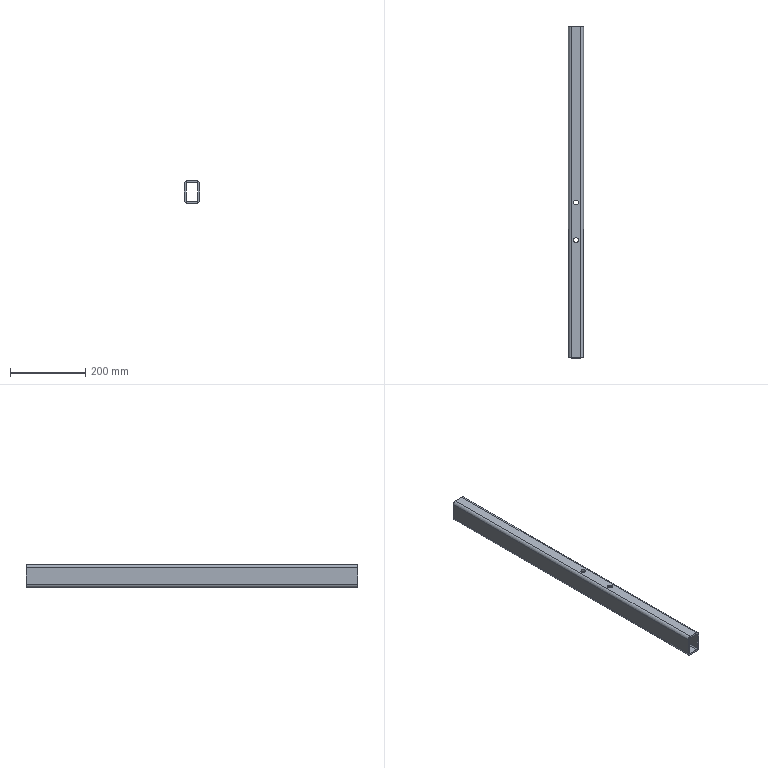Part | SolidWorks | features HoleWzd 1, WeldMemberFeat 1, WeldmentFeature 1 | 1 solid | 26 faces | box 40 x 884 x 60 mm | volume 751210 mm3 | cylinder 16 | plane 10 | commonest cylinder face diameters 13 x8 6 x4 16 x4
STEP:
#1=CARTESIAN_POINT('',(-6.5,314.,-30.));
#2=VERTEX_POINT('',#1);
#3=CARTESIAN_POINT('',(6.5,314.,-30.));
#4=VERTEX_POINT('',#3);
#5=CARTESIAN_POINT('',(0.,314.,-30.));
#6=DIRECTION('',(0.,0.,1.));
#7=DIRECTION('',(1.,0.,0.));
#8=AXIS2_PLACEMENT_3D('',#5,#6,#7);
#9=CIRCLE('',#8,6.5);
#10=EDGE_CURVE('',#2,#4,#9,.T.);
#11=ORIENTED_EDGE('',*,*,#10,.F.);
#12=CARTESIAN_POINT('',(-6.5,314.,-25.));
#13=VERTEX_POINT('',#12);
#14=CARTESIAN_POINT('',(-6.5,314.,30.));
#15=DIRECTION('',(0.,0.,1.));
#16=VECTOR('',#15,1000.);
#17=LINE('',#14,#16);
#18=EDGE_CURVE('',#2,#13,#17,.T.);
#19=ORIENTED_EDGE('',*,*,#18,.T.);
#20=CARTESIAN_POINT('',(6.5,314.,-25.));
#21=VERTEX_POINT('',#20);
#22=CARTESIAN_POINT('',(0.,314.,-25.));
#23=DIRECTION('',(0.,0.,1.));
#24=DIRECTION('',(1.,0.,0.));
#25=AXIS2_PLACEMENT_3D('',#22,#23,#24);
#26=CIRCLE('',#25,6.5);
#27=EDGE_CURVE('',#13,#21,#26,.T.);
#28=ORIENTED_EDGE('',*,*,#27,.T.);
#29=CARTESIAN_POINT('',(6.5,314.,30.));
#30=DIRECTION('',(0.,0.,1.));
#31=VECTOR('',#30,1000.);
#32=LINE('',#29,#31);
#33=EDGE_CURVE('',#4,#21,#32,.T.);
#34=ORIENTED_EDGE('',*,*,#33,.F.);
#35=EDGE_LOOP('',(#11,#19,#28,#34));
#36=FACE_OUTER_BOUND('',#35,.T.);
#37=CARTESIAN_POINT('',(0.,314.,30.));
#38=DIRECTION('',(0.,0.,1.));
#39=DIRECTION('',(1.,0.,0.));
#40=AXIS2_PLACEMENT_3D('',#37,#38,#39);
#41=CYLINDRICAL_SURFACE('',#40,6.5);
#42=ADVANCED_FACE('',(#36),#41,.F.);
#43=CARTESIAN_POINT('',(6.5,314.,25.));
#44=VERTEX_POINT('',#43);
#45=CARTESIAN_POINT('',(-6.5,314.,25.));
#46=VERTEX_POINT('',#45);
#47=CARTESIAN_POINT('',(0.,314.,25.));
#48=DIRECTION('',(0.,0.,-1.));
#49=DIRECTION('',(-1.,0.,0.));
#50=AXIS2_PLACEMENT_3D('',#47,#48,#49);
#51=CIRCLE('',#50,6.5);
#52=EDGE_CURVE('',#44,#46,#51,.T.);
#53=ORIENTED_EDGE('',*,*,#52,.T.);
#54=CARTESIAN_POINT('',(-6.5,314.,30.));
#55=VERTEX_POINT('',#54);
#56=CARTESIAN_POINT('',(-6.5,314.,30.));
#57=DIRECTION('',(0.,0.,1.));
#58=VECTOR('',#57,1000.);
#59=LINE('',#56,#58);
#60=EDGE_CURVE('',#46,#55,#59,.T.);
#61=ORIENTED_EDGE('',*,*,#60,.T.);
#62=CARTESIAN_POINT('',(6.5,314.,30.));
#63=VERTEX_POINT('',#62);
#64=CARTESIAN_POINT('',(0.,314.,30.));
#65=DIRECTION('',(0.,0.,1.));
#66=DIRECTION('',(1.,0.,0.));
#67=AXIS2_PLACEMENT_3D('',#64,#65,#66);
#68=CIRCLE('',#67,6.5);
#69=EDGE_CURVE('',#55,#63,#68,.T.);
#70=ORIENTED_EDGE('',*,*,#69,.T.);
#71=CARTESIAN_POINT('',(6.5,314.,30.));
#72=DIRECTION('',(0.,0.,1.));
#73=VECTOR('',#72,1000.);
#74=LINE('',#71,#73);
#75=EDGE_CURVE('',#44,#63,#74,.T.);
#76=ORIENTED_EDGE('',*,*,#75,.F.);
#77=EDGE_LOOP('',(#53,#61,#70,#76));
#78=FACE_OUTER_BOUND('',#77,.T.);
#79=CARTESIAN_POINT('',(0.,314.,30.));
#80=DIRECTION('',(0.,0.,1.));
#81=DIRECTION('',(1.,0.,0.));
#82=AXIS2_PLACEMENT_3D('',#79,#80,#81);
#83=CYLINDRICAL_SURFACE('',#82,6.5);
#84=ADVANCED_FACE('',(#78),#83,.F.);
#85=CARTESIAN_POINT('',(6.5,414.,25.));
#86=VERTEX_POINT('',#85);
#87=CARTESIAN_POINT('',(-6.5,414.,25.));
#88=VERTEX_POINT('',#87);
#89=CARTESIAN_POINT('',(0.,414.,25.));
#90=DIRECTION('',(0.,0.,-1.));
#91=DIRECTION('',(-1.,0.,0.));
#92=AXIS2_PLACEMENT_3D('',#89,#90,#91);
#93=CIRCLE('',#92,6.5);
#94=EDGE_CURVE('',#86,#88,#93,.T.);
#95=ORIENTED_EDGE('',*,*,#94,.T.);
#96=CARTESIAN_POINT('',(-6.5,414.,30.));
#97=VERTEX_POINT('',#96);
#98=CARTESIAN_POINT('',(-6.5,414.,30.));
#99=DIRECTION('',(0.,0.,1.));
#100=VECTOR('',#99,1000.);
#101=LINE('',#98,#100);
#102=EDGE_CURVE('',#88,#97,#101,.T.);
#103=ORIENTED_EDGE('',*,*,#102,.T.);
#104=CARTESIAN_POINT('',(6.5,414.,30.));
#105=VERTEX_POINT('',#104);
#106=CARTESIAN_POINT('',(0.,414.,30.));
#107=DIRECTION('',(0.,0.,1.));
#108=DIRECTION('',(1.,0.,0.));
#109=AXIS2_PLACEMENT_3D('',#106,#107,#108);
#110=CIRCLE('',#109,6.5);
#111=EDGE_CURVE('',#97,#105,#110,.T.);
#112=ORIENTED_EDGE('',*,*,#111,.T.);
#113=CARTESIAN_POINT('',(6.5,414.,30.));
#114=DIRECTION('',(0.,0.,1.));
#115=VECTOR('',#114,1000.);
#116=LINE('',#113,#115);
#117=EDGE_CURVE('',#86,#105,#116,.T.);
#118=ORIENTED_EDGE('',*,*,#117,.F.);
#119=EDGE_LOOP('',(#95,#103,#112,#118));
#120=FACE_OUTER_BOUND('',#119,.T.);
#121=CARTESIAN_POINT('',(0.,414.,30.));
#122=DIRECTION('',(0.,0.,1.));
#123=DIRECTION('',(1.,0.,0.));
#124=AXIS2_PLACEMENT_3D('',#121,#122,#123);
#125=CYLINDRICAL_SURFACE('',#124,6.5);
#126=ADVANCED_FACE('',(#120),#125,.F.);
#127=CARTESIAN_POINT('',(-6.5,414.,-30.));
#128=VERTEX_POINT('',#127);
#129=CARTESIAN_POINT('',(6.5,414.,-30.));
#130=VERTEX_POINT('',#129);
#131=CARTESIAN_POINT('',(0.,414.,-30.));
#132=DIRECTION('',(0.,0.,1.));
#133=DIRECTION('',(1.,0.,0.));
#134=AXIS2_PLACEMENT_3D('',#131,#132,#133);
#135=CIRCLE('',#134,6.5);
#136=EDGE_CURVE('',#128,#130,#135,.T.);
#137=ORIENTED_EDGE('',*,*,#136,.F.);
#138=CARTESIAN_POINT('',(-6.5,414.,-25.));
#139=VERTEX_POINT('',#138);
#140=CARTESIAN_POINT('',(-6.5,414.,30.));
#141=DIRECTION('',(0.,0.,1.));
#142=VECTOR('',#141,1000.);
#143=LINE('',#140,#142);
#144=EDGE_CURVE('',#128,#139,#143,.T.);
#145=ORIENTED_EDGE('',*,*,#144,.T.);
#146=CARTESIAN_POINT('',(6.5,414.,-25.));
#147=VERTEX_POINT('',#146);
#148=CARTESIAN_POINT('',(0.,414.,-25.));
#149=DIRECTION('',(0.,0.,1.));
#150=DIRECTION('',(1.,0.,0.));
#151=AXIS2_PLACEMENT_3D('',#148,#149,#150);
#152=CIRCLE('',#151,6.5);
#153=EDGE_CURVE('',#139,#147,#152,.T.);
#154=ORIENTED_EDGE('',*,*,#153,.T.);
#155=CARTESIAN_POINT('',(6.5,414.,30.));
#156=DIRECTION('',(0.,0.,1.));
#157=VECTOR('',#156,1000.);
#158=LINE('',#155,#157);
#159=EDGE_CURVE('',#130,#147,#158,.T.);
#160=ORIENTED_EDGE('',*,*,#159,.F.);
#161=EDGE_LOOP('',(#137,#145,#154,#160));
#162=FACE_OUTER_BOUND('',#161,.T.);
#163=CARTESIAN_POINT('',(0.,414.,30.));
#164=DIRECTION('',(0.,0.,1.));
#165=DIRECTION('',(1.,0.,0.));
#166=AXIS2_PLACEMENT_3D('',#163,#164,#165);
#167=CYLINDRICAL_SURFACE('',#166,6.5);
#168=ADVANCED_FACE('',(#162),#167,.F.);
#169=CARTESIAN_POINT('',(-20.,0.,22.));
#170=VERTEX_POINT('',#169);
#171=CARTESIAN_POINT('',(-12.,0.,30.));
#172=VERTEX_POINT('',#171);
#173=CARTESIAN_POINT('',(-12.,0.,22.));
#174=DIRECTION('',(0.,1.,0.));
#175=DIRECTION('',(0.,0.,1.));
#176=AXIS2_PLACEMENT_3D('',#173,#174,#175);
#177=CIRCLE('',#176,8.);
#178=EDGE_CURVE('',#170,#172,#177,.T.);
#179=ORIENTED_EDGE('',*,*,#178,.T.);
#180=CARTESIAN_POINT('',(-12.,884.,30.));
#181=VERTEX_POINT('',#180);
#182=CARTESIAN_POINT('',(-12.,884.,30.));
#183=DIRECTION('',(0.,-1.,0.));
#184=VECTOR('',#183,1000.);
#185=LINE('',#182,#184);
#186=EDGE_CURVE('',#181,#172,#185,.T.);
#187=ORIENTED_EDGE('',*,*,#186,.F.);
#188=CARTESIAN_POINT('',(-20.,884.,22.));
#189=VERTEX_POINT('',#188);
#190=CARTESIAN_POINT('',(-12.,884.,22.));
#191=DIRECTION('',(0.,1.,0.));
#192=DIRECTION('',(0.,0.,1.));
#193=AXIS2_PLACEMENT_3D('',#190,#191,#192);
#194=CIRCLE('',#193,8.);
#195=EDGE_CURVE('',#189,#181,#194,.T.);
#196=ORIENTED_EDGE('',*,*,#195,.F.);
#197=CARTESIAN_POINT('',(-20.,884.,22.));
#198=DIRECTION('',(0.,-1.,0.));
#199=VECTOR('',#198,1000.);
#200=LINE('',#197,#199);
#201=EDGE_CURVE('',#189,#170,#200,.T.);
#202=ORIENTED_EDGE('',*,*,#201,.T.);
#203=EDGE_LOOP('',(#179,#187,#196,#202));
#204=FACE_OUTER_BOUND('',#203,.T.);
#205=CARTESIAN_POINT('',(-12.,884.,22.));
#206=DIRECTION('',(0.,-1.,0.));
#207=DIRECTION('',(0.,0.,-1.));
#208=AXIS2_PLACEMENT_3D('',#205,#206,#207);
#209=CYLINDRICAL_SURFACE('',#208,8.);
#210=ADVANCED_FACE('',(#204),#209,.T.);
#211=CARTESIAN_POINT('',(0.,314.,30.));
#212=DIRECTION('',(0.,0.,1.));
#213=DIRECTION('',(1.,0.,0.));
#214=AXIS2_PLACEMENT_3D('',#211,#212,#213);
#215=CIRCLE('',#214,6.5);
#216=EDGE_CURVE('',#63,#55,#215,.T.);
#217=ORIENTED_EDGE('',*,*,#216,.F.);
#218=ORIENTED_EDGE('',*,*,#69,.F.);
#219=EDGE_LOOP('',(#217,#218));
#220=FACE_BOUND('',#219,.T.);
#221=CARTESIAN_POINT('',(0.,414.,30.));
#222=DIRECTION('',(0.,0.,1.));
#223=DIRECTION('',(1.,0.,0.));
#224=AXIS2_PLACEMENT_3D('',#221,#222,#223);
#225=CIRCLE('',#224,6.5);
#226=EDGE_CURVE('',#105,#97,#225,.T.);
#227=ORIENTED_EDGE('',*,*,#226,.F.);
#228=ORIENTED_EDGE('',*,*,#111,.F.);
#229=EDGE_LOOP('',(#227,#228));
#230=FACE_BOUND('',#229,.T.);
#231=CARTESIAN_POINT('',(12.,0.,30.));
#232=VERTEX_POINT('',#231);
#233=CARTESIAN_POINT('',(-12.,0.,30.));
#234=DIRECTION('',(1.,0.,0.));
#235=VECTOR('',#234,1000.);
#236=LINE('',#233,#235);
#237=EDGE_CURVE('',#172,#232,#236,.T.);
#238=ORIENTED_EDGE('',*,*,#237,.T.);
#239=CARTESIAN_POINT('',(12.,884.,30.));
#240=VERTEX_POINT('',#239);
#241=CARTESIAN_POINT('',(12.,884.,30.));
#242=DIRECTION('',(0.,-1.,0.));
#243=VECTOR('',#242,1000.);
#244=LINE('',#241,#243);
#245=EDGE_CURVE('',#240,#232,#244,.T.);
#246=ORIENTED_EDGE('',*,*,#245,.F.);
#247=CARTESIAN_POINT('',(-12.,884.,30.));
#248=DIRECTION('',(1.,0.,0.));
#249=VECTOR('',#248,1000.);
#250=LINE('',#247,#249);
#251=EDGE_CURVE('',#181,#240,#250,.T.);
#252=ORIENTED_EDGE('',*,*,#251,.F.);
#253=ORIENTED_EDGE('',*,*,#186,.T.);
#254=EDGE_LOOP('',(#238,#246,#252,#253));
#255=FACE_OUTER_BOUND('',#254,.T.);
#256=CARTESIAN_POINT('',(-12.,884.,30.));
#257=DIRECTION('',(0.,0.,-1.));
#258=DIRECTION('',(-1.,0.,0.));
#259=AXIS2_PLACEMENT_3D('',#256,#257,#258);
#260=PLANE('',#259);
#261=ADVANCED_FACE('',(#220,#230,#255),#260,.F.);
#262=CARTESIAN_POINT('',(20.,0.,22.));
#263=VERTEX_POINT('',#262);
#264=CARTESIAN_POINT('',(12.,0.,22.));
#265=DIRECTION('',(0.,1.,0.));
#266=DIRECTION('',(0.,0.,1.));
#267=AXIS2_PLACEMENT_3D('',#264,#265,#266);
#268=CIRCLE('',#267,8.);
#269=EDGE_CURVE('',#232,#263,#268,.T.);
#270=ORIENTED_EDGE('',*,*,#269,.T.);
#271=CARTESIAN_POINT('',(20.,884.,22.));
#272=VERTEX_POINT('',#271);
#273=CARTESIAN_POINT('',(20.,884.,22.));
#274=DIRECTION('',(0.,-1.,0.));
#275=VECTOR('',#274,1000.);
#276=LINE('',#273,#275);
#277=EDGE_CURVE('',#272,#263,#276,.T.);
#278=ORIENTED_EDGE('',*,*,#277,.F.);
#279=CARTESIAN_POINT('',(12.,884.,22.));
#280=DIRECTION('',(0.,1.,0.));
#281=DIRECTION('',(0.,0.,1.));
#282=AXIS2_PLACEMENT_3D('',#279,#280,#281);
#283=CIRCLE('',#282,8.);
#284=EDGE_CURVE('',#240,#272,#283,.T.);
#285=ORIENTED_EDGE('',*,*,#284,.F.);
#286=ORIENTED_EDGE('',*,*,#245,.T.);
#287=EDGE_LOOP('',(#270,#278,#285,#286));
#288=FACE_OUTER_BOUND('',#287,.T.);
#289=CARTESIAN_POINT('',(12.,884.,22.));
#290=DIRECTION('',(0.,-1.,0.));
#291=DIRECTION('',(0.,0.,-1.));
#292=AXIS2_PLACEMENT_3D('',#289,#290,#291);
#293=CYLINDRICAL_SURFACE('',#292,8.);
#294=ADVANCED_FACE('',(#288),#293,.T.);
#295=CARTESIAN_POINT('',(20.,0.,-22.));
#296=VERTEX_POINT('',#295);
#297=CARTESIAN_POINT('',(20.,0.,-22.));
#298=DIRECTION('',(0.,0.,-1.));
#299=VECTOR('',#298,1000.);
#300=LINE('',#297,#299);
#301=EDGE_CURVE('',#263,#296,#300,.T.);
#302=ORIENTED_EDGE('',*,*,#301,.T.);
#303=CARTESIAN_POINT('',(20.,884.,-22.));
#304=VERTEX_POINT('',#303);
#305=CARTESIAN_POINT('',(20.,884.,-22.));
#306=DIRECTION('',(0.,-1.,0.));
#307=VECTOR('',#306,1000.);
#308=LINE('',#305,#307);
#309=EDGE_CURVE('',#304,#296,#308,.T.);
#310=ORIENTED_EDGE('',*,*,#309,.F.);
#311=CARTESIAN_POINT('',(20.,884.,-22.));
#312=DIRECTION('',(0.,0.,-1.));
#313=VECTOR('',#312,1000.);
#314=LINE('',#311,#313);
#315=EDGE_CURVE('',#272,#304,#314,.T.);
#316=ORIENTED_EDGE('',*,*,#315,.F.);
#317=ORIENTED_EDGE('',*,*,#277,.T.);
#318=EDGE_LOOP('',(#302,#310,#316,#317));
#319=FACE_OUTER_BOUND('',#318,.T.);
#320=CARTESIAN_POINT('',(20.,884.,-22.));
#321=DIRECTION('',(-1.,0.,0.));
#322=DIRECTION('',(0.,0.,1.));
#323=AXIS2_PLACEMENT_3D('',#320,#321,#322);
#324=PLANE('',#323);
#325=ADVANCED_FACE('',(#319),#324,.F.);
#326=CARTESIAN_POINT('',(12.,0.,-30.));
#327=VERTEX_POINT('',#326);
#328=CARTESIAN_POINT('',(12.,0.,-22.));
#329=DIRECTION('',(0.,1.,0.));
#330=DIRECTION('',(0.,0.,1.));
#331=AXIS2_PLACEMENT_3D('',#328,#329,#330);
#332=CIRCLE('',#331,8.);
#333=EDGE_CURVE('',#296,#327,#332,.T.);
#334=ORIENTED_EDGE('',*,*,#333,.T.);
#335=CARTESIAN_POINT('',(12.,884.,-30.));
#336=VERTEX_POINT('',#335);
#337=CARTESIAN_POINT('',(12.,884.,-30.));
#338=DIRECTION('',(0.,-1.,0.));
#339=VECTOR('',#338,1000.);
#340=LINE('',#337,#339);
#341=EDGE_CURVE('',#336,#327,#340,.T.);
#342=ORIENTED_EDGE('',*,*,#341,.F.);
#343=CARTESIAN_POINT('',(12.,884.,-22.));
#344=DIRECTION('',(0.,1.,0.));
#345=DIRECTION('',(0.,0.,1.));
#346=AXIS2_PLACEMENT_3D('',#343,#344,#345);
#347=CIRCLE('',#346,8.);
#348=EDGE_CURVE('',#304,#336,#347,.T.);
#349=ORIENTED_EDGE('',*,*,#348,.F.);
#350=ORIENTED_EDGE('',*,*,#309,.T.);
#351=EDGE_LOOP('',(#334,#342,#349,#350));
#352=FACE_OUTER_BOUND('',#351,.T.);
#353=CARTESIAN_POINT('',(12.,884.,-22.));
#354=DIRECTION('',(0.,-1.,0.));
#355=DIRECTION('',(0.,0.,-1.));
#356=AXIS2_PLACEMENT_3D('',#353,#354,#355);
#357=CYLINDRICAL_SURFACE('',#356,8.);
#358=ADVANCED_FACE('',(#352),#357,.T.);
#359=CARTESIAN_POINT('',(0.,314.,-30.));
#360=DIRECTION('',(0.,0.,1.));
#361=DIRECTION('',(1.,0.,0.));
#362=AXIS2_PLACEMENT_3D('',#359,#360,#361);
#363=CIRCLE('',#362,6.5);
#364=EDGE_CURVE('',#4,#2,#363,.T.);
#365=ORIENTED_EDGE('',*,*,#364,.T.);
#366=ORIENTED_EDGE('',*,*,#10,.T.);
#367=EDGE_LOOP('',(#365,#366));
#368=FACE_BOUND('',#367,.T.);
#369=CARTESIAN_POINT('',(0.,414.,-30.));
#370=DIRECTION('',(0.,0.,1.));
#371=DIRECTION('',(1.,0.,0.));
#372=AXIS2_PLACEMENT_3D('',#369,#370,#371);
#373=CIRCLE('',#372,6.5);
#374=EDGE_CURVE('',#130,#128,#373,.T.);
#375=ORIENTED_EDGE('',*,*,#374,.T.);
#376=ORIENTED_EDGE('',*,*,#136,.T.);
#377=EDGE_LOOP('',(#375,#376));
#378=FACE_BOUND('',#377,.T.);
#379=CARTESIAN_POINT('',(-12.,0.,-30.));
#380=VERTEX_POINT('',#379);
#381=CARTESIAN_POINT('',(12.,0.,-30.));
#382=DIRECTION('',(-1.,0.,0.));
#383=VECTOR('',#382,1000.);
#384=LINE('',#381,#383);
#385=EDGE_CURVE('',#327,#380,#384,.T.);
#386=ORIENTED_EDGE('',*,*,#385,.T.);
#387=CARTESIAN_POINT('',(-12.,884.,-30.));
#388=VERTEX_POINT('',#387);
#389=CARTESIAN_POINT('',(-12.,884.,-30.));
#390=DIRECTION('',(0.,-1.,0.));
#391=VECTOR('',#390,1000.);
#392=LINE('',#389,#391);
#393=EDGE_CURVE('',#388,#380,#392,.T.);
#394=ORIENTED_EDGE('',*,*,#393,.F.);
#395=CARTESIAN_POINT('',(12.,884.,-30.));
#396=DIRECTION('',(-1.,0.,0.));
#397=VECTOR('',#396,1000.);
#398=LINE('',#395,#397);
#399=EDGE_CURVE('',#336,#388,#398,.T.);
#400=ORIENTED_EDGE('',*,*,#399,.F.);
#401=ORIENTED_EDGE('',*,*,#341,.T.);
#402=EDGE_LOOP('',(#386,#394,#400,#401));
#403=FACE_OUTER_BOUND('',#402,.T.);
#404=CARTESIAN_POINT('',(12.,884.,-30.));
#405=DIRECTION('',(0.,0.,1.));
#406=DIRECTION('',(1.,0.,0.));
#407=AXIS2_PLACEMENT_3D('',#404,#405,#406);
#408=PLANE('',#407);
#409=ADVANCED_FACE('',(#368,#378,#403),#408,.F.);
#410=CARTESIAN_POINT('',(-20.,0.,-22.));
#411=VERTEX_POINT('',#410);
#412=CARTESIAN_POINT('',(-12.,0.,-22.));
#413=DIRECTION('',(0.,1.,0.));
#414=DIRECTION('',(0.,0.,1.));
#415=AXIS2_PLACEMENT_3D('',#412,#413,#414);
#416=CIRCLE('',#415,8.);
#417=EDGE_CURVE('',#380,#411,#416,.T.);
#418=ORIENTED_EDGE('',*,*,#417,.T.);
#419=CARTESIAN_POINT('',(-20.,884.,-22.));
#420=VERTEX_POINT('',#419);
#421=CARTESIAN_POINT('',(-20.,884.,-22.));
#422=DIRECTION('',(0.,-1.,0.));
#423=VECTOR('',#422,1000.);
#424=LINE('',#421,#423);
#425=EDGE_CURVE('',#420,#411,#424,.T.);
#426=ORIENTED_EDGE('',*,*,#425,.F.);
#427=CARTESIAN_POINT('',(-12.,884.,-22.));
#428=DIRECTION('',(0.,1.,0.));
#429=DIRECTION('',(0.,0.,1.));
#430=AXIS2_PLACEMENT_3D('',#427,#428,#429);
#431=CIRCLE('',#430,8.);
#432=EDGE_CURVE('',#388,#420,#431,.T.);
#433=ORIENTED_EDGE('',*,*,#432,.F.);
#434=ORIENTED_EDGE('',*,*,#393,.T.);
#435=EDGE_LOOP('',(#418,#426,#433,#434));
#436=FACE_OUTER_BOUND('',#435,.T.);
#437=CARTESIAN_POINT('',(-12.,884.,-22.));
#438=DIRECTION('',(0.,-1.,0.));
#439=DIRECTION('',(0.,0.,-1.));
#440=AXIS2_PLACEMENT_3D('',#437,#438,#439);
#441=CYLINDRICAL_SURFACE('',#440,8.);
#442=ADVANCED_FACE('',(#436),#441,.T.);
#443=CARTESIAN_POINT('',(12.,0.,25.));
#444=VERTEX_POINT('',#443);
#445=CARTESIAN_POINT('',(15.,0.,22.));
#446=VERTEX_POINT('',#445);
#447=CARTESIAN_POINT('',(12.,0.,22.));
#448=DIRECTION('',(0.,1.,0.));
#449=DIRECTION('',(0.,0.,1.));
#450=AXIS2_PLACEMENT_3D('',#447,#448,#449);
#451=CIRCLE('',#450,3.);
#452=EDGE_CURVE('',#444,#446,#451,.T.);
#453=ORIENTED_EDGE('',*,*,#452,.F.);
#454=CARTESIAN_POINT('',(12.,884.,25.));
#455=VERTEX_POINT('',#454);
#456=CARTESIAN_POINT('',(12.,884.,25.));
#457=DIRECTION('',(0.,-1.,0.));
#458=VECTOR('',#457,1000.);
#459=LINE('',#456,#458);
#460=EDGE_CURVE('',#455,#444,#459,.T.);
#461=ORIENTED_EDGE('',*,*,#460,.F.);
#462=CARTESIAN_POINT('',(15.,884.,22.));
#463=VERTEX_POINT('',#462);
#464=CARTESIAN_POINT('',(12.,884.,22.));
#465=DIRECTION('',(0.,1.,0.));
#466=DIRECTION('',(0.,0.,1.));
#467=AXIS2_PLACEMENT_3D('',#464,#465,#466);
#468=CIRCLE('',#467,3.);
#469=EDGE_CURVE('',#455,#463,#468,.T.);
#470=ORIENTED_EDGE('',*,*,#469,.T.);
#471=CARTESIAN_POINT('',(15.,884.,22.));
#472=DIRECTION('',(0.,-1.,0.));
#473=VECTOR('',#472,1000.);
#474=LINE('',#471,#473);
#475=EDGE_CURVE('',#463,#446,#474,.T.);
#476=ORIENTED_EDGE('',*,*,#475,.T.);
#477=EDGE_LOOP('',(#453,#461,#470,#476));
#478=FACE_OUTER_BOUND('',#477,.T.);
#479=CARTESIAN_POINT('',(12.,884.,22.));
#480=DIRECTION('',(0.,-1.,0.));
#481=DIRECTION('',(0.,0.,-1.));
#482=AXIS2_PLACEMENT_3D('',#479,#480,#481);
#483=CYLINDRICAL_SURFACE('',#482,3.);
#484=ADVANCED_FACE('',(#478),#483,.F.);
#485=ORIENTED_EDGE('',*,*,#52,.F.);
#486=CARTESIAN_POINT('',(0.,314.,25.));
#487=DIRECTION('',(0.,0.,-1.));
#488=DIRECTION('',(-1.,0.,0.));
#489=AXIS2_PLACEMENT_3D('',#486,#487,#488);
#490=CIRCLE('',#489,6.5);
#491=EDGE_CURVE('',#46,#44,#490,.T.);
#492=ORIENTED_EDGE('',*,*,#491,.F.);
#493=EDGE_LOOP('',(#485,#492));
#494=FACE_BOUND('',#493,.T.);
#495=ORIENTED_EDGE('',*,*,#94,.F.);
#496=CARTESIAN_POINT('',(0.,414.,25.));
#497=DIRECTION('',(0.,0.,-1.));
#498=DIRECTION('',(-1.,0.,0.));
#499=AXIS2_PLACEMENT_3D('',#496,#497,#498);
#500=CIRCLE('',#499,6.5);
#501=EDGE_CURVE('',#88,#86,#500,.T.);
#502=ORIENTED_EDGE('',*,*,#501,.F.);
#503=EDGE_LOOP('',(#495,#502));
#504=FACE_BOUND('',#503,.T.);
#505=CARTESIAN_POINT('',(-12.,0.,25.));
#506=VERTEX_POINT('',#505);
#507=CARTESIAN_POINT('',(-12.,0.,25.));
#508=DIRECTION('',(1.,0.,0.));
#509=VECTOR('',#508,1000.);
#510=LINE('',#507,#509);
#511=EDGE_CURVE('',#506,#444,#510,.T.);
#512=ORIENTED_EDGE('',*,*,#511,.F.);
#513=CARTESIAN_POINT('',(-12.,884.,25.));
#514=VERTEX_POINT('',#513);
#515=CARTESIAN_POINT('',(-12.,884.,25.));
#516=DIRECTION('',(0.,-1.,0.));
#517=VECTOR('',#516,1000.);
#518=LINE('',#515,#517);
#519=EDGE_CURVE('',#514,#506,#518,.T.);
#520=ORIENTED_EDGE('',*,*,#519,.F.);
#521=CARTESIAN_POINT('',(-12.,884.,25.));
#522=DIRECTION('',(1.,0.,0.));
#523=VECTOR('',#522,1000.);
#524=LINE('',#521,#523);
#525=EDGE_CURVE('',#514,#455,#524,.T.);
#526=ORIENTED_EDGE('',*,*,#525,.T.);
#527=ORIENTED_EDGE('',*,*,#460,.T.);
#528=EDGE_LOOP('',(#512,#520,#526,#527));
#529=FACE_OUTER_BOUND('',#528,.T.);
#530=CARTESIAN_POINT('',(-12.,884.,25.));
#531=DIRECTION('',(0.,0.,-1.));
#532=DIRECTION('',(-1.,0.,0.));
#533=AXIS2_PLACEMENT_3D('',#530,#531,#532);
#534=PLANE('',#533);
#535=ADVANCED_FACE('',(#494,#504,#529),#534,.T.);
#536=CARTESIAN_POINT('',(-15.,0.,22.));
#537=VERTEX_POINT('',#536);
#538=CARTESIAN_POINT('',(-12.,0.,22.));
#539=DIRECTION('',(0.,1.,0.));
#540=DIRECTION('',(0.,0.,1.));
#541=AXIS2_PLACEMENT_3D('',#538,#539,#540);
#542=CIRCLE('',#541,3.);
#543=EDGE_CURVE('',#537,#506,#542,.T.);
#544=ORIENTED_EDGE('',*,*,#543,.F.);
#545=CARTESIAN_POINT('',(-15.,884.,22.));
#546=VERTEX_POINT('',#545);
#547=CARTESIAN_POINT('',(-15.,884.,22.));
#548=DIRECTION('',(0.,-1.,0.));
#549=VECTOR('',#548,1000.);
#550=LINE('',#547,#549);
#551=EDGE_CURVE('',#546,#537,#550,.T.);
#552=ORIENTED_EDGE('',*,*,#551,.F.);
#553=CARTESIAN_POINT('',(-12.,884.,22.));
#554=DIRECTION('',(0.,1.,0.));
#555=DIRECTION('',(0.,0.,1.));
#556=AXIS2_PLACEMENT_3D('',#553,#554,#555);
#557=CIRCLE('',#556,3.);
#558=EDGE_CURVE('',#546,#514,#557,.T.);
#559=ORIENTED_EDGE('',*,*,#558,.T.);
#560=ORIENTED_EDGE('',*,*,#519,.T.);
#561=EDGE_LOOP('',(#544,#552,#559,#560));
#562=FACE_OUTER_BOUND('',#561,.T.);
#563=CARTESIAN_POINT('',(-12.,884.,22.));
#564=DIRECTION('',(0.,-1.,0.));
#565=DIRECTION('',(0.,0.,-1.));
#566=AXIS2_PLACEMENT_3D('',#563,#564,#565);
#567=CYLINDRICAL_SURFACE('',#566,3.);
#568=ADVANCED_FACE('',(#562),#567,.F.);
#569=CARTESIAN_POINT('',(-15.,0.,-22.));
#570=VERTEX_POINT('',#569);
#571=CARTESIAN_POINT('',(-15.,0.,22.));
#572=DIRECTION('',(0.,0.,1.));
#573=VECTOR('',#572,1000.);
#574=LINE('',#571,#573);
#575=EDGE_CURVE('',#570,#537,#574,.T.);
#576=ORIENTED_EDGE('',*,*,#575,.F.);
#577=CARTESIAN_POINT('',(-15.,884.,-22.));
#578=VERTEX_POINT('',#577);
#579=CARTESIAN_POINT('',(-15.,884.,-22.));
#580=DIRECTION('',(0.,-1.,0.));
#581=VECTOR('',#580,1000.);
#582=LINE('',#579,#581);
#583=EDGE_CURVE('',#578,#570,#582,.T.);
#584=ORIENTED_EDGE('',*,*,#583,.F.);
#585=CARTESIAN_POINT('',(-15.,884.,22.));
#586=DIRECTION('',(0.,0.,1.));
#587=VECTOR('',#586,1000.);
#588=LINE('',#585,#587);
#589=EDGE_CURVE('',#578,#546,#588,.T.);
#590=ORIENTED_EDGE('',*,*,#589,.T.);
#591=ORIENTED_EDGE('',*,*,#551,.T.);
#592=EDGE_LOOP('',(#576,#584,#590,#591));
#593=FACE_OUTER_BOUND('',#592,.T.);
#594=CARTESIAN_POINT('',(-15.,884.,22.));
#595=DIRECTION('',(1.,0.,0.));
#596=DIRECTION('',(0.,0.,-1.));
#597=AXIS2_PLACEMENT_3D('',#594,#595,#596);
#598=PLANE('',#597);
#599=ADVANCED_FACE('',(#593),#598,.T.);
#600=CARTESIAN_POINT('',(-12.,0.,-25.));
#601=VERTEX_POINT('',#600);
#602=CARTESIAN_POINT('',(-12.,0.,-22.));
#603=DIRECTION('',(0.,1.,0.));
#604=DIRECTION('',(0.,0.,1.));
#605=AXIS2_PLACEMENT_3D('',#602,#603,#604);
#606=CIRCLE('',#605,3.);
#607=EDGE_CURVE('',#601,#570,#606,.T.);
#608=ORIENTED_EDGE('',*,*,#607,.F.);
#609=CARTESIAN_POINT('',(-12.,884.,-25.));
#610=VERTEX_POINT('',#609);
#611=CARTESIAN_POINT('',(-12.,884.,-25.));
#612=DIRECTION('',(0.,-1.,0.));
#613=VECTOR('',#612,1000.);
#614=LINE('',#611,#613);
#615=EDGE_CURVE('',#610,#601,#614,.T.);
#616=ORIENTED_EDGE('',*,*,#615,.F.);
#617=CARTESIAN_POINT('',(-12.,884.,-22.));
#618=DIRECTION('',(0.,1.,0.));
#619=DIRECTION('',(0.,0.,1.));
#620=AXIS2_PLACEMENT_3D('',#617,#618,#619);
#621=CIRCLE('',#620,3.);
#622=EDGE_CURVE('',#610,#578,#621,.T.);
#623=ORIENTED_EDGE('',*,*,#622,.T.);
#624=ORIENTED_EDGE('',*,*,#583,.T.);
#625=EDGE_LOOP('',(#608,#616,#623,#624));
#626=FACE_OUTER_BOUND('',#625,.T.);
#627=CARTESIAN_POINT('',(-12.,884.,-22.));
#628=DIRECTION('',(0.,-1.,0.));
#629=DIRECTION('',(0.,0.,-1.));
#630=AXIS2_PLACEMENT_3D('',#627,#628,#629);
#631=CYLINDRICAL_SURFACE('',#630,3.);
#632=ADVANCED_FACE('',(#626),#631,.F.);
#633=CARTESIAN_POINT('',(0.,314.,-25.));
#634=DIRECTION('',(0.,0.,1.));
#635=DIRECTION('',(1.,0.,0.));
#636=AXIS2_PLACEMENT_3D('',#633,#634,#635);
#637=CIRCLE('',#636,6.5);
#638=EDGE_CURVE('',#21,#13,#637,.T.);
#639=ORIENTED_EDGE('',*,*,#638,.F.);
#640=ORIENTED_EDGE('',*,*,#27,.F.);
#641=EDGE_LOOP('',(#639,#640));
#642=FACE_BOUND('',#641,.T.);
#643=CARTESIAN_POINT('',(0.,414.,-25.));
#644=DIRECTION('',(0.,0.,1.));
#645=DIRECTION('',(1.,0.,0.));
#646=AXIS2_PLACEMENT_3D('',#643,#644,#645);
#647=CIRCLE('',#646,6.5);
#648=EDGE_CURVE('',#147,#139,#647,.T.);
#649=ORIENTED_EDGE('',*,*,#648,.F.);
#650=ORIENTED_EDGE('',*,*,#153,.F.);
#651=EDGE_LOOP('',(#649,#650));
#652=FACE_BOUND('',#651,.T.);
#653=CARTESIAN_POINT('',(12.,0.,-25.));
#654=VERTEX_POINT('',#653);
#655=CARTESIAN_POINT('',(12.,0.,-25.));
#656=DIRECTION('',(-1.,0.,0.));
#657=VECTOR('',#656,1000.);
#658=LINE('',#655,#657);
#659=EDGE_CURVE('',#654,#601,#658,.T.);
#660=ORIENTED_EDGE('',*,*,#659,.F.);
#661=CARTESIAN_POINT('',(12.,884.,-25.));
#662=VERTEX_POINT('',#661);
#663=CARTESIAN_POINT('',(12.,884.,-25.));
#664=DIRECTION('',(0.,-1.,0.));
#665=VECTOR('',#664,1000.);
#666=LINE('',#663,#665);
#667=EDGE_CURVE('',#662,#654,#666,.T.);
#668=ORIENTED_EDGE('',*,*,#667,.F.);
#669=CARTESIAN_POINT('',(12.,884.,-25.));
#670=DIRECTION('',(-1.,0.,0.));
#671=VECTOR('',#670,1000.);
#672=LINE('',#669,#671);
#673=EDGE_CURVE('',#662,#610,#672,.T.);
#674=ORIENTED_EDGE('',*,*,#673,.T.);
#675=ORIENTED_EDGE('',*,*,#615,.T.);
#676=EDGE_LOOP('',(#660,#668,#674,#675));
#677=FACE_OUTER_BOUND('',#676,.T.);
#678=CARTESIAN_POINT('',(12.,884.,-25.));
#679=DIRECTION('',(0.,0.,1.));
#680=DIRECTION('',(1.,0.,0.));
#681=AXIS2_PLACEMENT_3D('',#678,#679,#680);
#682=PLANE('',#681);
#683=ADVANCED_FACE('',(#642,#652,#677),#682,.T.);
#684=CARTESIAN_POINT('',(15.,0.,-22.));
#685=VERTEX_POINT('',#684);
#686=CARTESIAN_POINT('',(12.,0.,-22.));
#687=DIRECTION('',(0.,1.,0.));
#688=DIRECTION('',(0.,0.,1.));
#689=AXIS2_PLACEMENT_3D('',#686,#687,#688);
#690=CIRCLE('',#689,3.);
#691=EDGE_CURVE('',#685,#654,#690,.T.);
#692=ORIENTED_EDGE('',*,*,#691,.F.);
#693=CARTESIAN_POINT('',(15.,884.,-22.));
#694=VERTEX_POINT('',#693);
#695=CARTESIAN_POINT('',(15.,884.,-22.));
#696=DIRECTION('',(0.,-1.,0.));
#697=VECTOR('',#696,1000.);
#698=LINE('',#695,#697);
#699=EDGE_CURVE('',#694,#685,#698,.T.);
#700=ORIENTED_EDGE('',*,*,#699,.F.);
#701=CARTESIAN_POINT('',(12.,884.,-22.));
#702=DIRECTION('',(0.,1.,0.));
#703=DIRECTION('',(0.,0.,1.));
#704=AXIS2_PLACEMENT_3D('',#701,#702,#703);
#705=CIRCLE('',#704,3.);
#706=EDGE_CURVE('',#694,#662,#705,.T.);
#707=ORIENTED_EDGE('',*,*,#706,.T.);
#708=ORIENTED_EDGE('',*,*,#667,.T.);
#709=EDGE_LOOP('',(#692,#700,#707,#708));
#710=FACE_OUTER_BOUND('',#709,.T.);
#711=CARTESIAN_POINT('',(12.,884.,-22.));
#712=DIRECTION('',(0.,-1.,0.));
#713=DIRECTION('',(0.,0.,-1.));
#714=AXIS2_PLACEMENT_3D('',#711,#712,#713);
#715=CYLINDRICAL_SURFACE('',#714,3.);
#716=ADVANCED_FACE('',(#710),#715,.F.);
#717=CARTESIAN_POINT('',(15.,0.,-22.));
#718=DIRECTION('',(0.,0.,-1.));
#719=VECTOR('',#718,1000.);
#720=LINE('',#717,#719);
#721=EDGE_CURVE('',#446,#685,#720,.T.);
#722=ORIENTED_EDGE('',*,*,#721,.F.);
#723=ORIENTED_EDGE('',*,*,#475,.F.);
#724=CARTESIAN_POINT('',(15.,884.,-22.));
#725=DIRECTION('',(0.,0.,-1.));
#726=VECTOR('',#725,1000.);
#727=LINE('',#724,#726);
#728=EDGE_CURVE('',#463,#694,#727,.T.);
#729=ORIENTED_EDGE('',*,*,#728,.T.);
#730=ORIENTED_EDGE('',*,*,#699,.T.);
#731=EDGE_LOOP('',(#722,#723,#729,#730));
#732=FACE_OUTER_BOUND('',#731,.T.);
#733=CARTESIAN_POINT('',(15.,884.,-22.));
#734=DIRECTION('',(-1.,0.,0.));
#735=DIRECTION('',(0.,0.,1.));
#736=AXIS2_PLACEMENT_3D('',#733,#734,#735);
#737=PLANE('',#736);
#738=ADVANCED_FACE('',(#732),#737,.T.);
#739=CARTESIAN_POINT('',(-20.,0.,22.));
#740=DIRECTION('',(0.,0.,1.));
#741=VECTOR('',#740,1000.);
#742=LINE('',#739,#741);
#743=EDGE_CURVE('',#411,#170,#742,.T.);
#744=ORIENTED_EDGE('',*,*,#743,.T.);
#745=ORIENTED_EDGE('',*,*,#201,.F.);
#746=CARTESIAN_POINT('',(-20.,884.,22.));
#747=DIRECTION('',(0.,0.,1.));
#748=VECTOR('',#747,1000.);
#749=LINE('',#746,#748);
#750=EDGE_CURVE('',#420,#189,#749,.T.);
#751=ORIENTED_EDGE('',*,*,#750,.F.);
#752=ORIENTED_EDGE('',*,*,#425,.T.);
#753=EDGE_LOOP('',(#744,#745,#751,#752));
#754=FACE_OUTER_BOUND('',#753,.T.);
#755=CARTESIAN_POINT('',(-20.,884.,22.));
#756=DIRECTION('',(1.,0.,0.));
#757=DIRECTION('',(0.,0.,-1.));
#758=AXIS2_PLACEMENT_3D('',#755,#756,#757);
#759=PLANE('',#758);
#760=ADVANCED_FACE('',(#754),#759,.F.);
#761=ORIENTED_EDGE('',*,*,#469,.F.);
#762=ORIENTED_EDGE('',*,*,#525,.F.);
#763=ORIENTED_EDGE('',*,*,#558,.F.);
#764=ORIENTED_EDGE('',*,*,#589,.F.);
#765=ORIENTED_EDGE('',*,*,#622,.F.);
#766=ORIENTED_EDGE('',*,*,#673,.F.);
#767=ORIENTED_EDGE('',*,*,#706,.F.);
#768=ORIENTED_EDGE('',*,*,#728,.F.);
#769=EDGE_LOOP('',(#761,#762,#763,#764,#765,#766,#767,#768));
#770=FACE_BOUND('',#769,.T.);
#771=ORIENTED_EDGE('',*,*,#195,.T.);
#772=ORIENTED_EDGE('',*,*,#251,.T.);
#773=ORIENTED_EDGE('',*,*,#284,.T.);
#774=ORIENTED_EDGE('',*,*,#315,.T.);
#775=ORIENTED_EDGE('',*,*,#348,.T.);
#776=ORIENTED_EDGE('',*,*,#399,.T.);
#777=ORIENTED_EDGE('',*,*,#432,.T.);
#778=ORIENTED_EDGE('',*,*,#750,.T.);
#779=EDGE_LOOP('',(#771,#772,#773,#774,#775,#776,#777,#778));
#780=FACE_OUTER_BOUND('',#779,.T.);
#781=CARTESIAN_POINT('',(-12.,884.,22.));
#782=DIRECTION('',(0.,1.,0.));
#783=DIRECTION('',(0.,0.,1.));
#784=AXIS2_PLACEMENT_3D('',#781,#782,#783);
#785=PLANE('',#784);
#786=ADVANCED_FACE('',(#770,#780),#785,.T.);
#787=ORIENTED_EDGE('',*,*,#452,.T.);
#788=ORIENTED_EDGE('',*,*,#721,.T.);
#789=ORIENTED_EDGE('',*,*,#691,.T.);
#790=ORIENTED_EDGE('',*,*,#659,.T.);
#791=ORIENTED_EDGE('',*,*,#607,.T.);
#792=ORIENTED_EDGE('',*,*,#575,.T.);
#793=ORIENTED_EDGE('',*,*,#543,.T.);
#794=ORIENTED_EDGE('',*,*,#511,.T.);
#795=EDGE_LOOP('',(#787,#788,#789,#790,#791,#792,#793,#794));
#796=FACE_BOUND('',#795,.T.);
#797=ORIENTED_EDGE('',*,*,#178,.F.);
#798=ORIENTED_EDGE('',*,*,#743,.F.);
#799=ORIENTED_EDGE('',*,*,#417,.F.);
#800=ORIENTED_EDGE('',*,*,#385,.F.);
#801=ORIENTED_EDGE('',*,*,#333,.F.);
#802=ORIENTED_EDGE('',*,*,#301,.F.);
#803=ORIENTED_EDGE('',*,*,#269,.F.);
#804=ORIENTED_EDGE('',*,*,#237,.F.);
#805=EDGE_LOOP('',(#797,#798,#799,#800,#801,#802,#803,#804));
#806=FACE_OUTER_BOUND('',#805,.T.);
#807=CARTESIAN_POINT('',(-12.,0.,22.));
#808=DIRECTION('',(0.,1.,0.));
#809=DIRECTION('',(0.,0.,1.));
#810=AXIS2_PLACEMENT_3D('',#807,#808,#809);
#811=PLANE('',#810);
#812=ADVANCED_FACE('',(#796,#806),#811,.F.);
#813=ORIENTED_EDGE('',*,*,#144,.F.);
#814=ORIENTED_EDGE('',*,*,#374,.F.);
#815=ORIENTED_EDGE('',*,*,#159,.T.);
#816=ORIENTED_EDGE('',*,*,#648,.T.);
#817=EDGE_LOOP('',(#813,#814,#815,#816));
#818=FACE_OUTER_BOUND('',#817,.T.);
#819=CARTESIAN_POINT('',(0.,414.,30.));
#820=DIRECTION('',(0.,0.,1.));
#821=DIRECTION('',(1.,0.,0.));
#822=AXIS2_PLACEMENT_3D('',#819,#820,#821);
#823=CYLINDRICAL_SURFACE('',#822,6.5);
#824=ADVANCED_FACE('',(#818),#823,.F.);
#825=ORIENTED_EDGE('',*,*,#102,.F.);
#826=ORIENTED_EDGE('',*,*,#501,.T.);
#827=ORIENTED_EDGE('',*,*,#117,.T.);
#828=ORIENTED_EDGE('',*,*,#226,.T.);
#829=EDGE_LOOP('',(#825,#826,#827,#828));
#830=FACE_OUTER_BOUND('',#829,.T.);
#831=CARTESIAN_POINT('',(0.,414.,30.));
#832=DIRECTION('',(0.,0.,1.));
#833=DIRECTION('',(1.,0.,0.));
#834=AXIS2_PLACEMENT_3D('',#831,#832,#833);
#835=CYLINDRICAL_SURFACE('',#834,6.5);
#836=ADVANCED_FACE('',(#830),#835,.F.);
#837=ORIENTED_EDGE('',*,*,#60,.F.);
#838=ORIENTED_EDGE('',*,*,#491,.T.);
#839=ORIENTED_EDGE('',*,*,#75,.T.);
#840=ORIENTED_EDGE('',*,*,#216,.T.);
#841=EDGE_LOOP('',(#837,#838,#839,#840));
#842=FACE_OUTER_BOUND('',#841,.T.);
#843=CARTESIAN_POINT('',(0.,314.,30.));
#844=DIRECTION('',(0.,0.,1.));
#845=DIRECTION('',(1.,0.,0.));
#846=AXIS2_PLACEMENT_3D('',#843,#844,#845);
#847=CYLINDRICAL_SURFACE('',#846,6.5);
#848=ADVANCED_FACE('',(#842),#847,.F.);
#849=ORIENTED_EDGE('',*,*,#18,.F.);
#850=ORIENTED_EDGE('',*,*,#364,.F.);
#851=ORIENTED_EDGE('',*,*,#33,.T.);
#852=ORIENTED_EDGE('',*,*,#638,.T.);
#853=EDGE_LOOP('',(#849,#850,#851,#852));
#854=FACE_OUTER_BOUND('',#853,.T.);
#855=CARTESIAN_POINT('',(0.,314.,30.));
#856=DIRECTION('',(0.,0.,1.));
#857=DIRECTION('',(1.,0.,0.));
#858=AXIS2_PLACEMENT_3D('',#855,#856,#857);
#859=CYLINDRICAL_SURFACE('',#858,6.5);
#860=ADVANCED_FACE('',(#854),#859,.F.);
#861=CLOSED_SHELL('',(#42,#84,#126,#168,#210,#261,#294,#325,#358,#409,#442,#484,#535,#568,#599,#632,#683,#716,#738,#760,#786,#812,#824,#836,#848,#860));
#862=MANIFOLD_SOLID_BREP('',#861);
#863=CARTESIAN_POINT('',(0.,0.,0.));
#864=DIRECTION('',(0.,0.,1.));
#865=DIRECTION('',(1.,0.,0.));
#866=AXIS2_PLACEMENT_3D('',#863,#864,#865);
#867=(LENGTH_UNIT()NAMED_UNIT(*)SI_UNIT(.MILLI.,.METRE.));
#868=UNCERTAINTY_MEASURE_WITH_UNIT(LENGTH_MEASURE(0.00001),#867,'','');
#869=(NAMED_UNIT(*)PLANE_ANGLE_UNIT()SI_UNIT($,.RADIAN.));
#870=(NAMED_UNIT(*)SI_UNIT($,.STERADIAN.)SOLID_ANGLE_UNIT());
#871=(GEOMETRIC_REPRESENTATION_CONTEXT(3)GLOBAL_UNCERTAINTY_ASSIGNED_CONTEXT((#868))GLOBAL_UNIT_ASSIGNED_CONTEXT((#867,#869,#870))REPRESENTATION_CONTEXT('',''));
#872=ADVANCED_BREP_SHAPE_REPRESENTATION('',(#862,#866),#871);